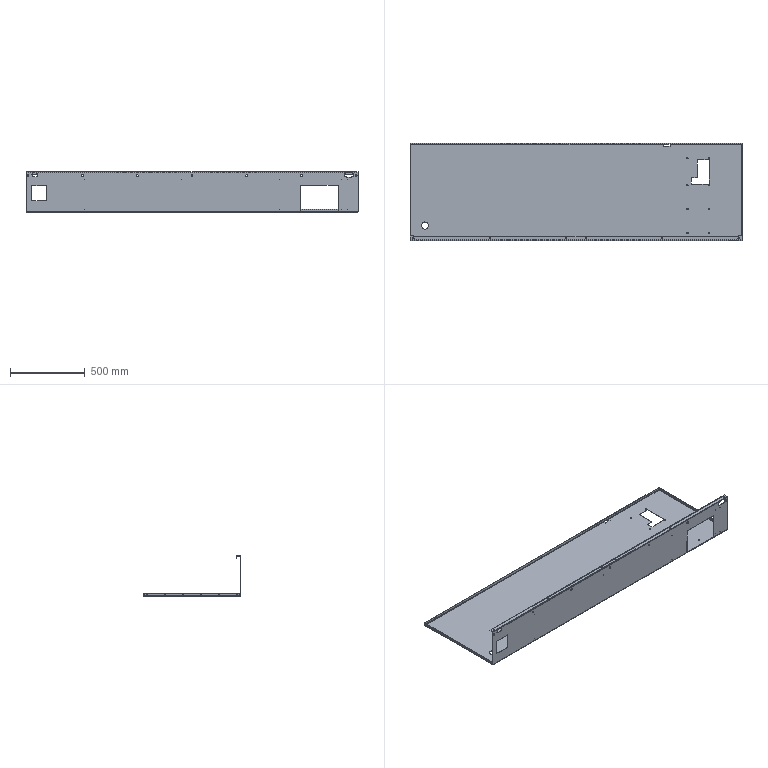Part | NX | features solid 2 | 1 solid | 188 faces | box 2215 x 648 x 270 mm | volume 4207771 mm3 | cylinder 108 | plane 80 | commonest cylinder face diameters 9.2 x28 6 x24 1 x18 12 x14 4 x6 7 x6